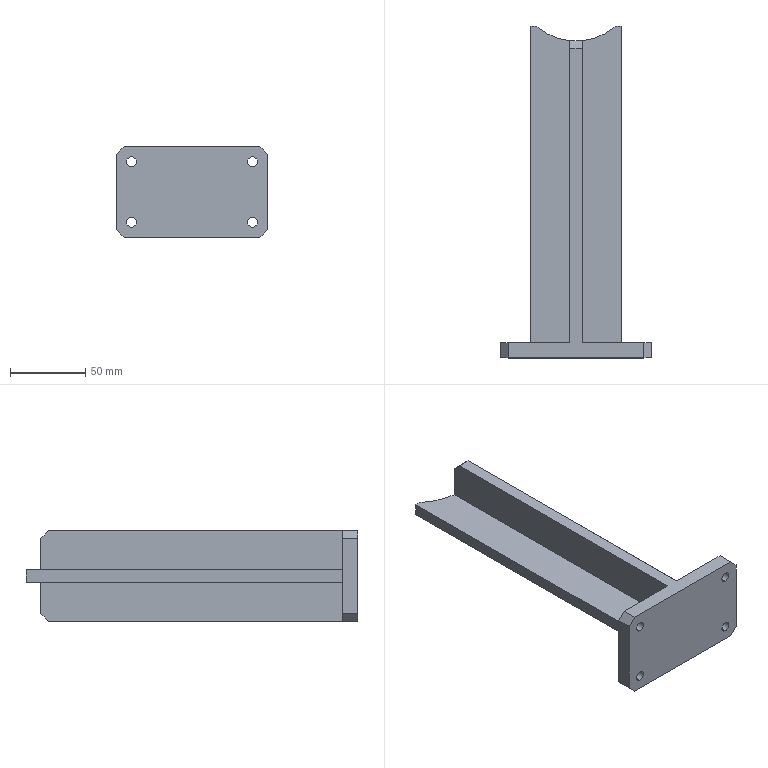Part | STEP file | Tube support base-front end | 1 solid | 36 faces | box 100 x 220 x 60 mm | volume 239052 mm3 | plane 23 | cylinder 11 | cone 2 | commonest cylinder face diameters 6.6 x8 10 x2 80 x1